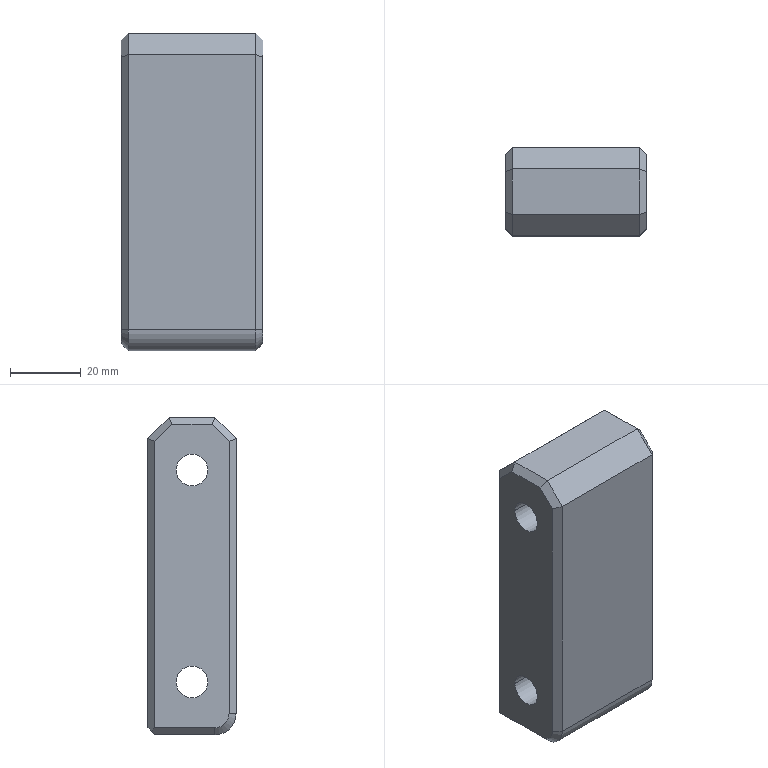Part | Creo | 1 solid | 34 faces | box 40 x 25 x 90 mm | volume 80599 mm3 | plane 23 | cylinder 9 | cone 2 | commonest cylinder face diameters 9 x4 14 x4 12 x1
STEP:
#1=CARTESIAN_POINT('',(294.5,48.167,78.));
#2=VERTEX_POINT('',#1);
#3=CARTESIAN_POINT('',(294.5,52.995,73.172));
#4=VERTEX_POINT('',#3);
#5=CARTESIAN_POINT('',(294.5,48.167,78.));
#6=DIRECTION('',(0.,0.7071,-0.7071));
#7=VECTOR('',#6,6.828);
#8=LINE('',#5,#7);
#9=EDGE_CURVE('',#2,#4,#8,.T.);
#10=ORIENTED_EDGE('',*,*,#9,.F.);
#11=CARTESIAN_POINT('',(294.5,36.824,78.));
#12=VERTEX_POINT('',#11);
#13=CARTESIAN_POINT('',(294.5,48.167,78.));
#14=DIRECTION('',(0.,-1.,0.));
#15=VECTOR('',#14,11.343);
#16=LINE('',#13,#15);
#17=EDGE_CURVE('',#2,#12,#16,.T.);
#18=ORIENTED_EDGE('',*,*,#17,.T.);
#19=CARTESIAN_POINT('',(294.5,31.995,73.172));
#20=VERTEX_POINT('',#19);
#21=CARTESIAN_POINT('',(294.5,31.995,73.172));
#22=DIRECTION('',(0.,0.7071,0.7071));
#23=VECTOR('',#22,6.828);
#24=LINE('',#21,#23);
#25=EDGE_CURVE('',#20,#12,#24,.T.);
#26=ORIENTED_EDGE('',*,*,#25,.F.);
#27=CARTESIAN_POINT('',(294.5,31.995,-4.));
#28=VERTEX_POINT('',#27);
#29=CARTESIAN_POINT('',(294.5,31.995,73.172));
#30=DIRECTION('',(0.,0.,-1.));
#31=VECTOR('',#30,77.172);
#32=LINE('',#29,#31);
#33=EDGE_CURVE('',#20,#28,#32,.T.);
#34=ORIENTED_EDGE('',*,*,#33,.T.);
#35=CARTESIAN_POINT('',(294.5,35.995,-8.));
#36=VERTEX_POINT('',#35);
#37=CARTESIAN_POINT('',(294.5,35.995,-4.));
#38=DIRECTION('',(-1.,0.,0.));
#39=DIRECTION('',(0.,0.,-1.));
#40=AXIS2_PLACEMENT_3D('',#37,#38,#39);
#41=CIRCLE('',#40,4.);
#42=EDGE_CURVE('',#36,#28,#41,.T.);
#43=ORIENTED_EDGE('',*,*,#42,.F.);
#44=CARTESIAN_POINT('',(294.5,52.995,-8.));
#45=VERTEX_POINT('',#44);
#46=CARTESIAN_POINT('',(294.5,35.995,-8.));
#47=DIRECTION('',(0.,1.,0.));
#48=VECTOR('',#47,17.);
#49=LINE('',#46,#48);
#50=EDGE_CURVE('',#36,#45,#49,.T.);
#51=ORIENTED_EDGE('',*,*,#50,.T.);
#52=CARTESIAN_POINT('',(294.5,52.995,-8.));
#53=DIRECTION('',(0.,0.,1.));
#54=VECTOR('',#53,81.172);
#55=LINE('',#52,#54);
#56=EDGE_CURVE('',#45,#4,#55,.T.);
#57=ORIENTED_EDGE('',*,*,#56,.T.);
#58=EDGE_LOOP('',(#10,#18,#26,#34,#43,#51,#57));
#59=FACE_OUTER_BOUND('',#58,.F.);
#60=CARTESIAN_POINT('',(294.5,46.995,65.));
#61=VERTEX_POINT('',#60);
#62=CARTESIAN_POINT('',(294.5,37.995,65.));
#63=VERTEX_POINT('',#62);
#64=CARTESIAN_POINT('',(294.5,42.495,65.));
#65=DIRECTION('',(1.,0.,0.));
#66=DIRECTION('',(0.,1.,0.));
#67=AXIS2_PLACEMENT_3D('',#64,#65,#66);
#68=CIRCLE('',#67,4.5);
#69=EDGE_CURVE('',#61,#63,#68,.T.);
#70=ORIENTED_EDGE('',*,*,#69,.F.);
#71=CARTESIAN_POINT('',(294.5,42.495,65.));
#72=DIRECTION('',(1.,0.,0.));
#73=DIRECTION('',(0.,-1.,0.));
#74=AXIS2_PLACEMENT_3D('',#71,#72,#73);
#75=CIRCLE('',#74,4.5);
#76=EDGE_CURVE('',#63,#61,#75,.T.);
#77=ORIENTED_EDGE('',*,*,#76,.F.);
#78=EDGE_LOOP('',(#70,#77));
#79=FACE_BOUND('',#78,.F.);
#80=CARTESIAN_POINT('',(294.5,46.995,5.));
#81=VERTEX_POINT('',#80);
#82=CARTESIAN_POINT('',(294.5,37.995,5.));
#83=VERTEX_POINT('',#82);
#84=CARTESIAN_POINT('',(294.5,42.495,5.));
#85=DIRECTION('',(1.,0.,0.));
#86=DIRECTION('',(0.,1.,0.));
#87=AXIS2_PLACEMENT_3D('',#84,#85,#86);
#88=CIRCLE('',#87,4.5);
#89=EDGE_CURVE('',#81,#83,#88,.T.);
#90=ORIENTED_EDGE('',*,*,#89,.F.);
#91=CARTESIAN_POINT('',(294.5,42.495,5.));
#92=DIRECTION('',(1.,0.,0.));
#93=DIRECTION('',(0.,-1.,0.));
#94=AXIS2_PLACEMENT_3D('',#91,#92,#93);
#95=CIRCLE('',#94,4.5);
#96=EDGE_CURVE('',#83,#81,#95,.T.);
#97=ORIENTED_EDGE('',*,*,#96,.F.);
#98=EDGE_LOOP('',(#90,#97));
#99=FACE_BOUND('',#98,.F.);
#100=CARTESIAN_POINT('',(294.5,42.745,-10.));
#101=DIRECTION('',(-1.,0.,0.));
#102=DIRECTION('',(0.,0.,-1.));
#103=AXIS2_PLACEMENT_3D('',#100,#101,#102);
#104=PLANE('',#103);
#105=ADVANCED_FACE('',(#59,#79,#99),#104,.T.);
#106=ORIENTED_EDGE('',*,*,#69,.T.);
#107=CARTESIAN_POINT('',(325.5,37.995,65.));
#108=VERTEX_POINT('',#107);
#109=CARTESIAN_POINT('',(294.5,37.995,65.));
#110=DIRECTION('',(1.,0.,0.));
#111=VECTOR('',#110,31.);
#112=LINE('',#109,#111);
#113=EDGE_CURVE('',#63,#108,#112,.T.);
#114=ORIENTED_EDGE('',*,*,#113,.T.);
#115=CARTESIAN_POINT('',(325.5,46.995,65.));
#116=VERTEX_POINT('',#115);
#117=CARTESIAN_POINT('',(325.5,42.495,65.));
#118=DIRECTION('',(-1.,0.,0.));
#119=DIRECTION('',(0.,-1.,0.));
#120=AXIS2_PLACEMENT_3D('',#117,#118,#119);
#121=CIRCLE('',#120,4.5);
#122=EDGE_CURVE('',#108,#116,#121,.T.);
#123=ORIENTED_EDGE('',*,*,#122,.T.);
#124=CARTESIAN_POINT('',(294.5,46.995,65.));
#125=DIRECTION('',(1.,0.,0.));
#126=VECTOR('',#125,31.);
#127=LINE('',#124,#126);
#128=EDGE_CURVE('',#61,#116,#127,.T.);
#129=ORIENTED_EDGE('',*,*,#128,.F.);
#130=EDGE_LOOP('',(#106,#114,#123,#129));
#131=FACE_OUTER_BOUND('',#130,.F.);
#132=CARTESIAN_POINT('',(334.5,42.495,65.));
#133=DIRECTION('',(1.,0.,0.));
#134=DIRECTION('',(0.,1.,0.));
#135=AXIS2_PLACEMENT_3D('',#132,#133,#134);
#136=CYLINDRICAL_SURFACE('',#135,4.5);
#137=ADVANCED_FACE('',(#131),#136,.F.);
#138=ORIENTED_EDGE('',*,*,#76,.T.);
#139=ORIENTED_EDGE('',*,*,#128,.T.);
#140=CARTESIAN_POINT('',(325.5,42.495,65.));
#141=DIRECTION('',(-1.,0.,0.));
#142=DIRECTION('',(0.,1.,0.));
#143=AXIS2_PLACEMENT_3D('',#140,#141,#142);
#144=CIRCLE('',#143,4.5);
#145=EDGE_CURVE('',#116,#108,#144,.T.);
#146=ORIENTED_EDGE('',*,*,#145,.T.);
#147=ORIENTED_EDGE('',*,*,#113,.F.);
#148=EDGE_LOOP('',(#138,#139,#146,#147));
#149=FACE_OUTER_BOUND('',#148,.F.);
#150=CARTESIAN_POINT('',(334.5,42.495,65.));
#151=DIRECTION('',(1.,0.,0.));
#152=DIRECTION('',(0.,1.,0.));
#153=AXIS2_PLACEMENT_3D('',#150,#151,#152);
#154=CYLINDRICAL_SURFACE('',#153,4.5);
#155=ADVANCED_FACE('',(#149),#154,.F.);
#156=CARTESIAN_POINT('',(325.5,49.495,65.));
#157=VERTEX_POINT('',#156);
#158=CARTESIAN_POINT('',(325.5,35.495,65.));
#159=VERTEX_POINT('',#158);
#160=CARTESIAN_POINT('',(325.5,42.495,65.));
#161=DIRECTION('',(1.,0.,0.));
#162=DIRECTION('',(0.,1.,0.));
#163=AXIS2_PLACEMENT_3D('',#160,#161,#162);
#164=CIRCLE('',#163,7.);
#165=EDGE_CURVE('',#157,#159,#164,.T.);
#166=ORIENTED_EDGE('',*,*,#165,.F.);
#167=CARTESIAN_POINT('',(325.5,42.495,65.));
#168=DIRECTION('',(1.,0.,0.));
#169=DIRECTION('',(0.,-1.,0.));
#170=AXIS2_PLACEMENT_3D('',#167,#168,#169);
#171=CIRCLE('',#170,7.);
#172=EDGE_CURVE('',#159,#157,#171,.T.);
#173=ORIENTED_EDGE('',*,*,#172,.F.);
#174=EDGE_LOOP('',(#166,#173));
#175=FACE_OUTER_BOUND('',#174,.F.);
#176=ORIENTED_EDGE('',*,*,#145,.F.);
#177=ORIENTED_EDGE('',*,*,#122,.F.);
#178=EDGE_LOOP('',(#176,#177));
#179=FACE_BOUND('',#178,.F.);
#180=CARTESIAN_POINT('',(325.5,42.495,65.));
#181=DIRECTION('',(-1.,0.,0.));
#182=DIRECTION('',(0.,0.,1.));
#183=AXIS2_PLACEMENT_3D('',#180,#181,#182);
#184=PLANE('',#183);
#185=ADVANCED_FACE('',(#175,#179),#184,.F.);
#186=ORIENTED_EDGE('',*,*,#165,.T.);
#187=CARTESIAN_POINT('',(334.5,35.495,65.));
#188=VERTEX_POINT('',#187);
#189=CARTESIAN_POINT('',(334.5,35.495,65.));
#190=DIRECTION('',(-1.,0.,0.));
#191=VECTOR('',#190,9.);
#192=LINE('',#189,#191);
#193=EDGE_CURVE('',#188,#159,#192,.T.);
#194=ORIENTED_EDGE('',*,*,#193,.F.);
#195=CARTESIAN_POINT('',(334.5,49.495,65.));
#196=VERTEX_POINT('',#195);
#197=CARTESIAN_POINT('',(334.5,42.495,65.));
#198=DIRECTION('',(-1.,0.,0.));
#199=DIRECTION('',(0.,-1.,0.));
#200=AXIS2_PLACEMENT_3D('',#197,#198,#199);
#201=CIRCLE('',#200,7.);
#202=EDGE_CURVE('',#188,#196,#201,.T.);
#203=ORIENTED_EDGE('',*,*,#202,.T.);
#204=CARTESIAN_POINT('',(334.5,49.495,65.));
#205=DIRECTION('',(-1.,0.,0.));
#206=VECTOR('',#205,9.);
#207=LINE('',#204,#206);
#208=EDGE_CURVE('',#196,#157,#207,.T.);
#209=ORIENTED_EDGE('',*,*,#208,.T.);
#210=EDGE_LOOP('',(#186,#194,#203,#209));
#211=FACE_OUTER_BOUND('',#210,.F.);
#212=CARTESIAN_POINT('',(334.5,42.495,65.));
#213=DIRECTION('',(-1.,0.,0.));
#214=DIRECTION('',(0.,1.,0.));
#215=AXIS2_PLACEMENT_3D('',#212,#213,#214);
#216=CYLINDRICAL_SURFACE('',#215,7.);
#217=ADVANCED_FACE('',(#211),#216,.F.);
#218=ORIENTED_EDGE('',*,*,#172,.T.);
#219=ORIENTED_EDGE('',*,*,#208,.F.);
#220=CARTESIAN_POINT('',(334.5,42.495,65.));
#221=DIRECTION('',(-1.,0.,0.));
#222=DIRECTION('',(0.,1.,0.));
#223=AXIS2_PLACEMENT_3D('',#220,#221,#222);
#224=CIRCLE('',#223,7.);
#225=EDGE_CURVE('',#196,#188,#224,.T.);
#226=ORIENTED_EDGE('',*,*,#225,.T.);
#227=ORIENTED_EDGE('',*,*,#193,.T.);
#228=EDGE_LOOP('',(#218,#219,#226,#227));
#229=FACE_OUTER_BOUND('',#228,.F.);
#230=CARTESIAN_POINT('',(334.5,42.495,65.));
#231=DIRECTION('',(-1.,0.,0.));
#232=DIRECTION('',(0.,1.,0.));
#233=AXIS2_PLACEMENT_3D('',#230,#231,#232);
#234=CYLINDRICAL_SURFACE('',#233,7.);
#235=ADVANCED_FACE('',(#229),#234,.F.);
#236=CARTESIAN_POINT('',(334.5,52.995,73.172));
#237=VERTEX_POINT('',#236);
#238=CARTESIAN_POINT('',(334.5,48.167,78.));
#239=VERTEX_POINT('',#238);
#240=CARTESIAN_POINT('',(334.5,52.995,73.172));
#241=DIRECTION('',(0.,-0.7071,0.7071));
#242=VECTOR('',#241,6.828);
#243=LINE('',#240,#242);
#244=EDGE_CURVE('',#237,#239,#243,.T.);
#245=ORIENTED_EDGE('',*,*,#244,.F.);
#246=CARTESIAN_POINT('',(334.5,52.995,-8.));
#247=VERTEX_POINT('',#246);
#248=CARTESIAN_POINT('',(334.5,52.995,73.172));
#249=DIRECTION('',(0.,0.,-1.));
#250=VECTOR('',#249,81.172);
#251=LINE('',#248,#250);
#252=EDGE_CURVE('',#237,#247,#251,.T.);
#253=ORIENTED_EDGE('',*,*,#252,.T.);
#254=CARTESIAN_POINT('',(334.5,35.995,-8.));
#255=VERTEX_POINT('',#254);
#256=CARTESIAN_POINT('',(334.5,52.995,-8.));
#257=DIRECTION('',(0.,-1.,0.));
#258=VECTOR('',#257,17.);
#259=LINE('',#256,#258);
#260=EDGE_CURVE('',#247,#255,#259,.T.);
#261=ORIENTED_EDGE('',*,*,#260,.T.);
#262=CARTESIAN_POINT('',(334.5,31.995,-4.));
#263=VERTEX_POINT('',#262);
#264=CARTESIAN_POINT('',(334.5,35.995,-4.));
#265=DIRECTION('',(1.,0.,0.));
#266=DIRECTION('',(0.,-1.,0.));
#267=AXIS2_PLACEMENT_3D('',#264,#265,#266);
#268=CIRCLE('',#267,4.);
#269=EDGE_CURVE('',#263,#255,#268,.T.);
#270=ORIENTED_EDGE('',*,*,#269,.F.);
#271=CARTESIAN_POINT('',(334.5,31.995,73.172));
#272=VERTEX_POINT('',#271);
#273=CARTESIAN_POINT('',(334.5,31.995,-4.));
#274=DIRECTION('',(0.,0.,1.));
#275=VECTOR('',#274,77.172);
#276=LINE('',#273,#275);
#277=EDGE_CURVE('',#263,#272,#276,.T.);
#278=ORIENTED_EDGE('',*,*,#277,.T.);
#279=CARTESIAN_POINT('',(334.5,36.824,78.));
#280=VERTEX_POINT('',#279);
#281=CARTESIAN_POINT('',(334.5,36.824,78.));
#282=DIRECTION('',(0.,-0.7071,-0.7071));
#283=VECTOR('',#282,6.828);
#284=LINE('',#281,#283);
#285=EDGE_CURVE('',#280,#272,#284,.T.);
#286=ORIENTED_EDGE('',*,*,#285,.F.);
#287=CARTESIAN_POINT('',(334.5,36.824,78.));
#288=DIRECTION('',(0.,1.,0.));
#289=VECTOR('',#288,11.343);
#290=LINE('',#287,#289);
#291=EDGE_CURVE('',#280,#239,#290,.T.);
#292=ORIENTED_EDGE('',*,*,#291,.T.);
#293=EDGE_LOOP('',(#245,#253,#261,#270,#278,#286,#292));
#294=FACE_OUTER_BOUND('',#293,.F.);
#295=ORIENTED_EDGE('',*,*,#225,.F.);
#296=ORIENTED_EDGE('',*,*,#202,.F.);
#297=EDGE_LOOP('',(#295,#296));
#298=FACE_BOUND('',#297,.F.);
#299=CARTESIAN_POINT('',(334.5,49.495,5.));
#300=VERTEX_POINT('',#299);
#301=CARTESIAN_POINT('',(334.5,35.495,5.));
#302=VERTEX_POINT('',#301);
#303=CARTESIAN_POINT('',(334.5,42.495,5.));
#304=DIRECTION('',(-1.,0.,0.));
#305=DIRECTION('',(0.,1.,0.));
#306=AXIS2_PLACEMENT_3D('',#303,#304,#305);
#307=CIRCLE('',#306,7.);
#308=EDGE_CURVE('',#300,#302,#307,.T.);
#309=ORIENTED_EDGE('',*,*,#308,.F.);
#310=CARTESIAN_POINT('',(334.5,42.495,5.));
#311=DIRECTION('',(-1.,0.,0.));
#312=DIRECTION('',(0.,-1.,0.));
#313=AXIS2_PLACEMENT_3D('',#310,#311,#312);
#314=CIRCLE('',#313,7.);
#315=EDGE_CURVE('',#302,#300,#314,.T.);
#316=ORIENTED_EDGE('',*,*,#315,.F.);
#317=EDGE_LOOP('',(#309,#316));
#318=FACE_BOUND('',#317,.F.);
#319=CARTESIAN_POINT('',(334.5,42.745,-10.));
#320=DIRECTION('',(1.,0.,0.));
#321=DIRECTION('',(0.,0.,1.));
#322=AXIS2_PLACEMENT_3D('',#319,#320,#321);
#323=PLANE('',#322);
#324=ADVANCED_FACE('',(#294,#298,#318),#323,.T.);
#325=CARTESIAN_POINT('',(332.5,54.995,74.));
#326=VERTEX_POINT('',#325);
#327=CARTESIAN_POINT('',(332.5,54.995,74.));
#328=DIRECTION('',(0.6786,-0.6786,-0.2811));
#329=VECTOR('',#328,2.947);
#330=LINE('',#327,#329);
#331=EDGE_CURVE('',#326,#237,#330,.T.);
#332=ORIENTED_EDGE('',*,*,#331,.T.);
#333=ORIENTED_EDGE('',*,*,#244,.T.);
#334=CARTESIAN_POINT('',(332.5,48.995,80.));
#335=VERTEX_POINT('',#334);
#336=CARTESIAN_POINT('',(334.5,48.167,78.));
#337=DIRECTION('',(-0.6786,0.2811,0.6786));
#338=VECTOR('',#337,2.947);
#339=LINE('',#336,#338);
#340=EDGE_CURVE('',#239,#335,#339,.T.);
#341=ORIENTED_EDGE('',*,*,#340,.T.);
#342=CARTESIAN_POINT('',(332.5,54.995,74.));
#343=DIRECTION('',(0.,-0.7071,0.7071));
#344=VECTOR('',#343,8.485);
#345=LINE('',#342,#344);
#346=EDGE_CURVE('',#326,#335,#345,.T.);
#347=ORIENTED_EDGE('',*,*,#346,.F.);
#348=EDGE_LOOP('',(#332,#333,#341,#347));
#349=FACE_OUTER_BOUND('',#348,.F.);
#350=CARTESIAN_POINT('',(334.5,89.456,36.711));
#351=DIRECTION('',(0.7071,0.5,0.5));
#352=DIRECTION('',(0.,0.7071,-0.7071));
#353=AXIS2_PLACEMENT_3D('',#350,#351,#352);
#354=PLANE('',#353);
#355=ADVANCED_FACE('',(#349),#354,.T.);
#356=CARTESIAN_POINT('',(333.5,53.995,-9.));
#357=VERTEX_POINT('',#356);
#358=CARTESIAN_POINT('',(333.5,53.995,-9.));
#359=DIRECTION('',(0.5774,-0.5774,0.5774));
#360=VECTOR('',#359,1.732);
#361=LINE('',#358,#360);
#362=EDGE_CURVE('',#357,#247,#361,.T.);
#363=ORIENTED_EDGE('',*,*,#362,.T.);
#364=ORIENTED_EDGE('',*,*,#252,.F.);
#365=ORIENTED_EDGE('',*,*,#331,.F.);
#366=CARTESIAN_POINT('',(332.5,54.995,-8.));
#367=VERTEX_POINT('',#366);
#368=CARTESIAN_POINT('',(332.5,54.995,-8.));
#369=DIRECTION('',(0.,0.,1.));
#370=VECTOR('',#369,82.);
#371=LINE('',#368,#370);
#372=EDGE_CURVE('',#367,#326,#371,.T.);
#373=ORIENTED_EDGE('',*,*,#372,.F.);
#374=CARTESIAN_POINT('',(332.5,54.995,-8.));
#375=DIRECTION('',(0.5774,-0.5774,-0.5774));
#376=VECTOR('',#375,1.732);
#377=LINE('',#374,#376);
#378=EDGE_CURVE('',#367,#357,#377,.T.);
#379=ORIENTED_EDGE('',*,*,#378,.T.);
#380=EDGE_LOOP('',(#363,#364,#365,#373,#379));
#381=FACE_OUTER_BOUND('',#380,.F.);
#382=CARTESIAN_POINT('',(332.5,54.995,35.));
#383=DIRECTION('',(0.7071,0.7071,0.));
#384=DIRECTION('',(0.,0.,1.));
#385=AXIS2_PLACEMENT_3D('',#382,#383,#384);
#386=PLANE('',#385);
#387=ADVANCED_FACE('',(#381),#386,.T.);
#388=CARTESIAN_POINT('',(332.5,35.995,-10.));
#389=VERTEX_POINT('',#388);
#390=CARTESIAN_POINT('',(332.5,52.995,-10.));
#391=VERTEX_POINT('',#390);
#392=CARTESIAN_POINT('',(332.5,35.995,-10.));
#393=DIRECTION('',(0.,1.,0.));
#394=VECTOR('',#393,17.);
#395=LINE('',#392,#394);
#396=EDGE_CURVE('',#389,#391,#395,.T.);
#397=ORIENTED_EDGE('',*,*,#396,.F.);
#398=CARTESIAN_POINT('',(332.5,35.995,-10.));
#399=DIRECTION('',(0.7071,0.,0.7071));
#400=VECTOR('',#399,2.828);
#401=LINE('',#398,#400);
#402=EDGE_CURVE('',#389,#255,#401,.T.);
#403=ORIENTED_EDGE('',*,*,#402,.T.);
#404=ORIENTED_EDGE('',*,*,#260,.F.);
#405=ORIENTED_EDGE('',*,*,#362,.F.);
#406=CARTESIAN_POINT('',(333.5,53.995,-9.));
#407=DIRECTION('',(-0.5774,-0.5774,-0.5774));
#408=VECTOR('',#407,1.732);
#409=LINE('',#406,#408);
#410=EDGE_CURVE('',#357,#391,#409,.T.);
#411=ORIENTED_EDGE('',*,*,#410,.T.);
#412=EDGE_LOOP('',(#397,#403,#404,#405,#411));
#413=FACE_OUTER_BOUND('',#412,.F.);
#414=CARTESIAN_POINT('',(332.5,42.745,-10.));
#415=DIRECTION('',(-0.7071,0.,0.7071));
#416=DIRECTION('',(0.,-1.,0.));
#417=AXIS2_PLACEMENT_3D('',#414,#415,#416);
#418=PLANE('',#417);
#419=ADVANCED_FACE('',(#413),#418,.F.);
#420=CARTESIAN_POINT('',(296.5,52.995,-10.));
#421=VERTEX_POINT('',#420);
#422=CARTESIAN_POINT('',(296.5,35.995,-10.));
#423=VERTEX_POINT('',#422);
#424=CARTESIAN_POINT('',(296.5,52.995,-10.));
#425=DIRECTION('',(0.,-1.,0.));
#426=VECTOR('',#425,17.);
#427=LINE('',#424,#426);
#428=EDGE_CURVE('',#421,#423,#427,.T.);
#429=ORIENTED_EDGE('',*,*,#428,.T.);
#430=CARTESIAN_POINT('',(296.5,35.995,-10.));
#431=DIRECTION('',(1.,0.,0.));
#432=VECTOR('',#431,36.);
#433=LINE('',#430,#432);
#434=EDGE_CURVE('',#423,#389,#433,.T.);
#435=ORIENTED_EDGE('',*,*,#434,.T.);
#436=ORIENTED_EDGE('',*,*,#396,.T.);
#437=CARTESIAN_POINT('',(332.5,52.995,-10.));
#438=DIRECTION('',(-1.,0.,0.));
#439=VECTOR('',#438,36.);
#440=LINE('',#437,#439);
#441=EDGE_CURVE('',#391,#421,#440,.T.);
#442=ORIENTED_EDGE('',*,*,#441,.T.);
#443=EDGE_LOOP('',(#429,#435,#436,#442));
#444=FACE_OUTER_BOUND('',#443,.F.);
#445=CARTESIAN_POINT('',(318.5,42.745,-10.));
#446=DIRECTION('',(0.,0.,-1.));
#447=DIRECTION('',(1.,0.,0.));
#448=AXIS2_PLACEMENT_3D('',#445,#446,#447);
#449=PLANE('',#448);
#450=ADVANCED_FACE('',(#444),#449,.T.);
#451=CARTESIAN_POINT('',(295.5,53.995,-9.));
#452=VERTEX_POINT('',#451);
#453=CARTESIAN_POINT('',(294.5,52.995,-8.));
#454=DIRECTION('',(0.5774,0.5774,-0.5774));
#455=VECTOR('',#454,1.732);
#456=LINE('',#453,#455);
#457=EDGE_CURVE('',#45,#452,#456,.T.);
#458=ORIENTED_EDGE('',*,*,#457,.F.);
#459=ORIENTED_EDGE('',*,*,#50,.F.);
#460=CARTESIAN_POINT('',(294.5,35.995,-8.));
#461=DIRECTION('',(0.7071,0.,-0.7071));
#462=VECTOR('',#461,2.828);
#463=LINE('',#460,#462);
#464=EDGE_CURVE('',#36,#423,#463,.T.);
#465=ORIENTED_EDGE('',*,*,#464,.T.);
#466=ORIENTED_EDGE('',*,*,#428,.F.);
#467=CARTESIAN_POINT('',(296.5,52.995,-10.));
#468=DIRECTION('',(-0.5774,0.5774,0.5774));
#469=VECTOR('',#468,1.732);
#470=LINE('',#467,#469);
#471=EDGE_CURVE('',#421,#452,#470,.T.);
#472=ORIENTED_EDGE('',*,*,#471,.T.);
#473=EDGE_LOOP('',(#458,#459,#465,#466,#472));
#474=FACE_OUTER_BOUND('',#473,.F.);
#475=CARTESIAN_POINT('',(296.5,42.745,-10.));
#476=DIRECTION('',(0.7071,0.,0.7071));
#477=DIRECTION('',(0.,1.,0.));
#478=AXIS2_PLACEMENT_3D('',#475,#476,#477);
#479=PLANE('',#478);
#480=ADVANCED_FACE('',(#474),#479,.F.);
#481=CARTESIAN_POINT('',(296.5,54.995,74.));
#482=VERTEX_POINT('',#481);
#483=CARTESIAN_POINT('',(296.5,54.995,-8.));
#484=VERTEX_POINT('',#483);
#485=CARTESIAN_POINT('',(296.5,54.995,74.));
#486=DIRECTION('',(0.,0.,-1.));
#487=VECTOR('',#486,82.);
#488=LINE('',#485,#487);
#489=EDGE_CURVE('',#482,#484,#488,.T.);
#490=ORIENTED_EDGE('',*,*,#489,.F.);
#491=CARTESIAN_POINT('',(296.5,54.995,74.));
#492=DIRECTION('',(-0.6786,-0.6786,-0.2811));
#493=VECTOR('',#492,2.947);
#494=LINE('',#491,#493);
#495=EDGE_CURVE('',#482,#4,#494,.T.);
#496=ORIENTED_EDGE('',*,*,#495,.T.);
#497=ORIENTED_EDGE('',*,*,#56,.F.);
#498=ORIENTED_EDGE('',*,*,#457,.T.);
#499=CARTESIAN_POINT('',(295.5,53.995,-9.));
#500=DIRECTION('',(0.5774,0.5774,0.5774));
#501=VECTOR('',#500,1.732);
#502=LINE('',#499,#501);
#503=EDGE_CURVE('',#452,#484,#502,.T.);
#504=ORIENTED_EDGE('',*,*,#503,.T.);
#505=EDGE_LOOP('',(#490,#496,#497,#498,#504));
#506=FACE_OUTER_BOUND('',#505,.F.);
#507=CARTESIAN_POINT('',(294.5,52.995,-10.));
#508=DIRECTION('',(-0.7071,0.7071,0.));
#509=DIRECTION('',(0.,0.,1.));
#510=AXIS2_PLACEMENT_3D('',#507,#508,#509);
#511=PLANE('',#510);
#512=ADVANCED_FACE('',(#506),#511,.T.);
#513=ORIENTED_EDGE('',*,*,#372,.T.);
#514=CARTESIAN_POINT('',(332.5,54.995,74.));
#515=DIRECTION('',(-1.,0.,0.));
#516=VECTOR('',#515,36.);
#517=LINE('',#514,#516);
#518=EDGE_CURVE('',#326,#482,#517,.T.);
#519=ORIENTED_EDGE('',*,*,#518,.T.);
#520=ORIENTED_EDGE('',*,*,#489,.T.);
#521=CARTESIAN_POINT('',(296.5,54.995,-8.));
#522=DIRECTION('',(1.,0.,0.));
#523=VECTOR('',#522,36.);
#524=LINE('',#521,#523);
#525=EDGE_CURVE('',#484,#367,#524,.T.);
#526=ORIENTED_EDGE('',*,*,#525,.T.);
#527=EDGE_LOOP('',(#513,#519,#520,#526));
#528=FACE_OUTER_BOUND('',#527,.F.);
#529=CARTESIAN_POINT('',(318.5,54.995,35.));
#530=DIRECTION('',(0.,-1.,0.));
#531=DIRECTION('',(0.,0.,-1.));
#532=AXIS2_PLACEMENT_3D('',#529,#530,#531);
#533=PLANE('',#532);
#534=ADVANCED_FACE('',(#528),#533,.F.);
#535=CARTESIAN_POINT('',(296.5,48.995,80.));
#536=VERTEX_POINT('',#535);
#537=CARTESIAN_POINT('',(296.5,48.995,80.));
#538=DIRECTION('',(1.,0.,0.));
#539=VECTOR('',#538,36.);
#540=LINE('',#537,#539);
#541=EDGE_CURVE('',#536,#335,#540,.T.);
#542=ORIENTED_EDGE('',*,*,#541,.F.);
#543=CARTESIAN_POINT('',(296.5,48.995,80.));
#544=DIRECTION('',(0.,0.7071,-0.7071));
#545=VECTOR('',#544,8.485);
#546=LINE('',#543,#545);
#547=EDGE_CURVE('',#536,#482,#546,.T.);
#548=ORIENTED_EDGE('',*,*,#547,.T.);
#549=ORIENTED_EDGE('',*,*,#518,.F.);
#550=ORIENTED_EDGE('',*,*,#346,.T.);
#551=EDGE_LOOP('',(#542,#548,#549,#550));
#552=FACE_OUTER_BOUND('',#551,.F.);
#553=CARTESIAN_POINT('',(318.5,54.995,74.));
#554=DIRECTION('',(0.,-0.7071,-0.7071));
#555=DIRECTION('',(1.,0.,0.));
#556=AXIS2_PLACEMENT_3D('',#553,#554,#555);
#557=PLANE('',#556);
#558=ADVANCED_FACE('',(#552),#557,.F.);
#559=CARTESIAN_POINT('',(332.5,35.995,80.));
#560=VERTEX_POINT('',#559);
#561=CARTESIAN_POINT('',(296.5,35.995,80.));
#562=VERTEX_POINT('',#561);
#563=CARTESIAN_POINT('',(332.5,35.995,80.));
#564=DIRECTION('',(-1.,0.,0.));
#565=VECTOR('',#564,36.);
#566=LINE('',#563,#565);
#567=EDGE_CURVE('',#560,#562,#566,.T.);
#568=ORIENTED_EDGE('',*,*,#567,.T.);
#569=CARTESIAN_POINT('',(296.5,35.995,80.));
#570=DIRECTION('',(0.,1.,0.));
#571=VECTOR('',#570,13.);
#572=LINE('',#569,#571);
#573=EDGE_CURVE('',#562,#536,#572,.T.);
#574=ORIENTED_EDGE('',*,*,#573,.T.);
#575=ORIENTED_EDGE('',*,*,#541,.T.);
#576=CARTESIAN_POINT('',(332.5,48.995,80.));
#577=DIRECTION('',(0.,-1.,0.));
#578=VECTOR('',#577,13.);
#579=LINE('',#576,#578);
#580=EDGE_CURVE('',#335,#560,#579,.T.);
#581=ORIENTED_EDGE('',*,*,#580,.T.);
#582=EDGE_LOOP('',(#568,#574,#575,#581));
#583=FACE_OUTER_BOUND('',#582,.F.);
#584=CARTESIAN_POINT('',(318.5,42.745,80.));
#585=DIRECTION('',(0.,0.,-1.));
#586=DIRECTION('',(1.,0.,0.));
#587=AXIS2_PLACEMENT_3D('',#584,#585,#586);
#588=PLANE('',#587);
#589=ADVANCED_FACE('',(#583),#588,.F.);
#590=CARTESIAN_POINT('',(296.5,29.995,74.));
#591=VERTEX_POINT('',#590);
#592=CARTESIAN_POINT('',(332.5,29.995,74.));
#593=VERTEX_POINT('',#592);
#594=CARTESIAN_POINT('',(296.5,29.995,74.));
#595=DIRECTION('',(1.,0.,0.));
#596=VECTOR('',#595,36.);
#597=LINE('',#594,#596);
#598=EDGE_CURVE('',#591,#593,#597,.T.);
#599=ORIENTED_EDGE('',*,*,#598,.F.);
#600=CARTESIAN_POINT('',(296.5,29.995,74.));
#601=DIRECTION('',(0.,0.7071,0.7071));
#602=VECTOR('',#601,8.485);
#603=LINE('',#600,#602);
#604=EDGE_CURVE('',#591,#562,#603,.T.);
#605=ORIENTED_EDGE('',*,*,#604,.T.);
#606=ORIENTED_EDGE('',*,*,#567,.F.);
#607=CARTESIAN_POINT('',(332.5,35.995,80.));
#608=DIRECTION('',(0.,-0.7071,-0.7071));
#609=VECTOR('',#608,8.485);
#610=LINE('',#607,#609);
#611=EDGE_CURVE('',#560,#593,#610,.T.);
#612=ORIENTED_EDGE('',*,*,#611,.T.);
#613=EDGE_LOOP('',(#599,#605,#606,#612));
#614=FACE_OUTER_BOUND('',#613,.F.);
#615=CARTESIAN_POINT('',(318.5,35.995,80.));
#616=DIRECTION('',(0.,-0.7071,0.7071));
#617=DIRECTION('',(-1.,0.,0.));
#618=AXIS2_PLACEMENT_3D('',#615,#616,#617);
#619=PLANE('',#618);
#620=ADVANCED_FACE('',(#614),#619,.T.);
#621=CARTESIAN_POINT('',(332.5,29.995,-4.));
#622=VERTEX_POINT('',#621);
#623=CARTESIAN_POINT('',(296.5,29.995,-4.));
#624=VERTEX_POINT('',#623);
#625=CARTESIAN_POINT('',(332.5,29.995,-4.));
#626=DIRECTION('',(-1.,0.,0.));
#627=VECTOR('',#626,36.);
#628=LINE('',#625,#627);
#629=EDGE_CURVE('',#622,#624,#628,.T.);
#630=ORIENTED_EDGE('',*,*,#629,.T.);
#631=CARTESIAN_POINT('',(296.5,29.995,-4.));
#632=DIRECTION('',(0.,0.,1.));
#633=VECTOR('',#632,78.);
#634=LINE('',#631,#633);
#635=EDGE_CURVE('',#624,#591,#634,.T.);
#636=ORIENTED_EDGE('',*,*,#635,.T.);
#637=ORIENTED_EDGE('',*,*,#598,.T.);
#638=CARTESIAN_POINT('',(332.5,29.995,74.));
#639=DIRECTION('',(0.,0.,-1.));
#640=VECTOR('',#639,78.);
#641=LINE('',#638,#640);
#642=EDGE_CURVE('',#593,#622,#641,.T.);
#643=ORIENTED_EDGE('',*,*,#642,.T.);
#644=EDGE_LOOP('',(#630,#636,#637,#643));
#645=FACE_OUTER_BOUND('',#644,.F.);
#646=CARTESIAN_POINT('',(318.5,29.995,-10.));
#647=DIRECTION('',(0.,-1.,0.));
#648=DIRECTION('',(0.,0.,-1.));
#649=AXIS2_PLACEMENT_3D('',#646,#647,#648);
#650=PLANE('',#649);
#651=ADVANCED_FACE('',(#645),#650,.T.);
#652=ORIENTED_EDGE('',*,*,#434,.F.);
#653=CARTESIAN_POINT('',(296.5,35.995,-4.));
#654=DIRECTION('',(-1.,0.,0.));
#655=DIRECTION('',(0.,0.,-1.));
#656=AXIS2_PLACEMENT_3D('',#653,#654,#655);
#657=CIRCLE('',#656,6.);
#658=EDGE_CURVE('',#423,#624,#657,.T.);
#659=ORIENTED_EDGE('',*,*,#658,.T.);
#660=ORIENTED_EDGE('',*,*,#629,.F.);
#661=CARTESIAN_POINT('',(332.5,35.995,-4.));
#662=DIRECTION('',(1.,0.,0.));
#663=DIRECTION('',(0.,-1.,0.));
#664=AXIS2_PLACEMENT_3D('',#661,#662,#663);
#665=CIRCLE('',#664,6.);
#666=EDGE_CURVE('',#622,#389,#665,.T.);
#667=ORIENTED_EDGE('',*,*,#666,.T.);
#668=EDGE_LOOP('',(#652,#659,#660,#667));
#669=FACE_OUTER_BOUND('',#668,.F.);
#670=CARTESIAN_POINT('',(318.5,35.995,-4.));
#671=DIRECTION('',(-1.,0.,0.));
#672=DIRECTION('',(0.,0.,1.));
#673=AXIS2_PLACEMENT_3D('',#670,#671,#672);
#674=CYLINDRICAL_SURFACE('',#673,6.);
#675=ADVANCED_FACE('',(#669),#674,.T.);
#676=CARTESIAN_POINT('',(296.5,29.995,-4.));
#677=DIRECTION('',(-0.7071,0.7071,0.));
#678=VECTOR('',#677,2.828);
#679=LINE('',#676,#678);
#680=EDGE_CURVE('',#624,#28,#679,.T.);
#681=ORIENTED_EDGE('',*,*,#680,.F.);
#682=ORIENTED_EDGE('',*,*,#658,.F.);
#683=ORIENTED_EDGE('',*,*,#464,.F.);
#684=ORIENTED_EDGE('',*,*,#42,.T.);
#685=EDGE_LOOP('',(#681,#682,#683,#684));
#686=FACE_OUTER_BOUND('',#685,.F.);
#687=CARTESIAN_POINT('',(295.5,35.995,-4.));
#688=DIRECTION('',(1.,0.,0.));
#689=DIRECTION('',(0.,0.,-1.));
#690=AXIS2_PLACEMENT_3D('',#687,#688,#689);
#691=CONICAL_SURFACE('',#690,5.,45.);
#692=ADVANCED_FACE('',(#686),#691,.T.);
#693=CARTESIAN_POINT('',(294.5,31.995,73.172));
#694=DIRECTION('',(0.6786,-0.6786,0.2811));
#695=VECTOR('',#694,2.947);
#696=LINE('',#693,#695);
#697=EDGE_CURVE('',#20,#591,#696,.T.);
#698=ORIENTED_EDGE('',*,*,#697,.T.);
#699=ORIENTED_EDGE('',*,*,#635,.F.);
#700=ORIENTED_EDGE('',*,*,#680,.T.);
#701=ORIENTED_EDGE('',*,*,#33,.F.);
#702=EDGE_LOOP('',(#698,#699,#700,#701));
#703=FACE_OUTER_BOUND('',#702,.F.);
#704=CARTESIAN_POINT('',(296.5,29.995,-10.));
#705=DIRECTION('',(0.7071,0.7071,0.));
#706=DIRECTION('',(0.,0.,-1.));
#707=AXIS2_PLACEMENT_3D('',#704,#705,#706);
#708=PLANE('',#707);
#709=ADVANCED_FACE('',(#703),#708,.F.);
#710=CARTESIAN_POINT('',(296.5,35.995,80.));
#711=DIRECTION('',(-0.6786,0.2811,-0.6786));
#712=VECTOR('',#711,2.947);
#713=LINE('',#710,#712);
#714=EDGE_CURVE('',#562,#12,#713,.T.);
#715=ORIENTED_EDGE('',*,*,#714,.F.);
#716=ORIENTED_EDGE('',*,*,#604,.F.);
#717=ORIENTED_EDGE('',*,*,#697,.F.);
#718=ORIENTED_EDGE('',*,*,#25,.T.);
#719=EDGE_LOOP('',(#715,#716,#717,#718));
#720=FACE_OUTER_BOUND('',#719,.F.);
#721=CARTESIAN_POINT('',(294.5,-4.215,36.961));
#722=DIRECTION('',(0.7071,0.5,-0.5));
#723=DIRECTION('',(0.,0.7071,0.7071));
#724=AXIS2_PLACEMENT_3D('',#721,#722,#723);
#725=PLANE('',#724);
#726=ADVANCED_FACE('',(#720),#725,.F.);
#727=ORIENTED_EDGE('',*,*,#714,.T.);
#728=ORIENTED_EDGE('',*,*,#17,.F.);
#729=CARTESIAN_POINT('',(296.5,48.995,80.));
#730=DIRECTION('',(-0.6786,-0.2811,-0.6786));
#731=VECTOR('',#730,2.947);
#732=LINE('',#729,#731);
#733=EDGE_CURVE('',#536,#2,#732,.T.);
#734=ORIENTED_EDGE('',*,*,#733,.F.);
#735=ORIENTED_EDGE('',*,*,#573,.F.);
#736=EDGE_LOOP('',(#727,#728,#734,#735));
#737=FACE_OUTER_BOUND('',#736,.F.);
#738=CARTESIAN_POINT('',(294.5,42.745,78.));
#739=DIRECTION('',(-0.7071,0.,0.7071));
#740=DIRECTION('',(0.,-1.,0.));
#741=AXIS2_PLACEMENT_3D('',#738,#739,#740);
#742=PLANE('',#741);
#743=ADVANCED_FACE('',(#737),#742,.T.);
#744=ORIENTED_EDGE('',*,*,#733,.T.);
#745=ORIENTED_EDGE('',*,*,#9,.T.);
#746=ORIENTED_EDGE('',*,*,#495,.F.);
#747=ORIENTED_EDGE('',*,*,#547,.F.);
#748=EDGE_LOOP('',(#744,#745,#746,#747));
#749=FACE_OUTER_BOUND('',#748,.F.);
#750=CARTESIAN_POINT('',(294.5,89.456,36.711));
#751=DIRECTION('',(-0.7071,0.5,0.5));
#752=DIRECTION('',(0.,-0.7071,0.7071));
#753=AXIS2_PLACEMENT_3D('',#750,#751,#752);
#754=PLANE('',#753);
#755=ADVANCED_FACE('',(#749),#754,.T.);
#756=ORIENTED_EDGE('',*,*,#402,.F.);
#757=ORIENTED_EDGE('',*,*,#666,.F.);
#758=CARTESIAN_POINT('',(334.5,31.995,-4.));
#759=DIRECTION('',(-0.7071,-0.7071,0.));
#760=VECTOR('',#759,2.828);
#761=LINE('',#758,#760);
#762=EDGE_CURVE('',#263,#622,#761,.T.);
#763=ORIENTED_EDGE('',*,*,#762,.F.);
#764=ORIENTED_EDGE('',*,*,#269,.T.);
#765=EDGE_LOOP('',(#756,#757,#763,#764));
#766=FACE_OUTER_BOUND('',#765,.F.);
#767=CARTESIAN_POINT('',(333.5,35.995,-4.));
#768=DIRECTION('',(-1.,0.,0.));
#769=DIRECTION('',(0.,0.,1.));
#770=AXIS2_PLACEMENT_3D('',#767,#768,#769);
#771=CONICAL_SURFACE('',#770,5.,45.);
#772=ADVANCED_FACE('',(#766),#771,.T.);
#773=ORIENTED_EDGE('',*,*,#762,.T.);
#774=ORIENTED_EDGE('',*,*,#642,.F.);
#775=CARTESIAN_POINT('',(334.5,31.995,73.172));
#776=DIRECTION('',(-0.6786,-0.6786,0.2811));
#777=VECTOR('',#776,2.947);
#778=LINE('',#775,#777);
#779=EDGE_CURVE('',#272,#593,#778,.T.);
#780=ORIENTED_EDGE('',*,*,#779,.F.);
#781=ORIENTED_EDGE('',*,*,#277,.F.);
#782=EDGE_LOOP('',(#773,#774,#780,#781));
#783=FACE_OUTER_BOUND('',#782,.F.);
#784=CARTESIAN_POINT('',(332.5,29.995,-10.));
#785=DIRECTION('',(-0.7071,0.7071,0.));
#786=DIRECTION('',(0.,0.,1.));
#787=AXIS2_PLACEMENT_3D('',#784,#785,#786);
#788=PLANE('',#787);
#789=ADVANCED_FACE('',(#783),#788,.F.);
#790=ORIENTED_EDGE('',*,*,#779,.T.);
#791=ORIENTED_EDGE('',*,*,#611,.F.);
#792=CARTESIAN_POINT('',(334.5,36.824,78.));
#793=DIRECTION('',(-0.6786,-0.2811,0.6786));
#794=VECTOR('',#793,2.947);
#795=LINE('',#792,#794);
#796=EDGE_CURVE('',#280,#560,#795,.T.);
#797=ORIENTED_EDGE('',*,*,#796,.F.);
#798=ORIENTED_EDGE('',*,*,#285,.T.);
#799=EDGE_LOOP('',(#790,#791,#797,#798));
#800=FACE_OUTER_BOUND('',#799,.F.);
#801=CARTESIAN_POINT('',(334.5,-4.215,36.961));
#802=DIRECTION('',(-0.7071,0.5,-0.5));
#803=DIRECTION('',(0.,-0.7071,-0.7071));
#804=AXIS2_PLACEMENT_3D('',#801,#802,#803);
#805=PLANE('',#804);
#806=ADVANCED_FACE('',(#800),#805,.F.);
#807=ORIENTED_EDGE('',*,*,#796,.T.);
#808=ORIENTED_EDGE('',*,*,#580,.F.);
#809=ORIENTED_EDGE('',*,*,#340,.F.);
#810=ORIENTED_EDGE('',*,*,#291,.F.);
#811=EDGE_LOOP('',(#807,#808,#809,#810));
#812=FACE_OUTER_BOUND('',#811,.F.);
#813=CARTESIAN_POINT('',(332.5,42.745,80.));
#814=DIRECTION('',(0.7071,0.,0.7071));
#815=DIRECTION('',(0.,-1.,0.));
#816=AXIS2_PLACEMENT_3D('',#813,#814,#815);
#817=PLANE('',#816);
#818=ADVANCED_FACE('',(#812),#817,.T.);
#819=ORIENTED_EDGE('',*,*,#503,.F.);
#820=ORIENTED_EDGE('',*,*,#471,.F.);
#821=ORIENTED_EDGE('',*,*,#441,.F.);
#822=ORIENTED_EDGE('',*,*,#410,.F.);
#823=ORIENTED_EDGE('',*,*,#378,.F.);
#824=ORIENTED_EDGE('',*,*,#525,.F.);
#825=EDGE_LOOP('',(#819,#820,#821,#822,#823,#824));
#826=FACE_OUTER_BOUND('',#825,.F.);
#827=CARTESIAN_POINT('',(318.5,52.995,-10.));
#828=DIRECTION('',(0.,0.7071,-0.7071));
#829=DIRECTION('',(-1.,0.,0.));
#830=AXIS2_PLACEMENT_3D('',#827,#828,#829);
#831=PLANE('',#830);
#832=ADVANCED_FACE('',(#826),#831,.T.);
#833=CARTESIAN_POINT('',(325.5,35.495,5.));
#834=VERTEX_POINT('',#833);
#835=CARTESIAN_POINT('',(325.5,49.495,5.));
#836=VERTEX_POINT('',#835);
#837=CARTESIAN_POINT('',(325.5,42.495,5.));
#838=DIRECTION('',(1.,0.,0.));
#839=DIRECTION('',(0.,-1.,0.));
#840=AXIS2_PLACEMENT_3D('',#837,#838,#839);
#841=CIRCLE('',#840,7.);
#842=EDGE_CURVE('',#834,#836,#841,.T.);
#843=ORIENTED_EDGE('',*,*,#842,.T.);
#844=CARTESIAN_POINT('',(334.5,49.495,5.));
#845=DIRECTION('',(-1.,0.,0.));
#846=VECTOR('',#845,9.);
#847=LINE('',#844,#846);
#848=EDGE_CURVE('',#300,#836,#847,.T.);
#849=ORIENTED_EDGE('',*,*,#848,.F.);
#850=ORIENTED_EDGE('',*,*,#308,.T.);
#851=CARTESIAN_POINT('',(334.5,35.495,5.));
#852=DIRECTION('',(-1.,0.,0.));
#853=VECTOR('',#852,9.);
#854=LINE('',#851,#853);
#855=EDGE_CURVE('',#302,#834,#854,.T.);
#856=ORIENTED_EDGE('',*,*,#855,.T.);
#857=EDGE_LOOP('',(#843,#849,#850,#856));
#858=FACE_OUTER_BOUND('',#857,.F.);
#859=CARTESIAN_POINT('',(334.5,42.495,5.));
#860=DIRECTION('',(-1.,0.,0.));
#861=DIRECTION('',(0.,1.,0.));
#862=AXIS2_PLACEMENT_3D('',#859,#860,#861);
#863=CYLINDRICAL_SURFACE('',#862,7.);
#864=ADVANCED_FACE('',(#858),#863,.F.);
#865=CARTESIAN_POINT('',(325.5,42.495,5.));
#866=DIRECTION('',(1.,0.,0.));
#867=DIRECTION('',(0.,1.,0.));
#868=AXIS2_PLACEMENT_3D('',#865,#866,#867);
#869=CIRCLE('',#868,7.);
#870=EDGE_CURVE('',#836,#834,#869,.T.);
#871=ORIENTED_EDGE('',*,*,#870,.F.);
#872=ORIENTED_EDGE('',*,*,#842,.F.);
#873=EDGE_LOOP('',(#871,#872));
#874=FACE_OUTER_BOUND('',#873,.F.);
#875=CARTESIAN_POINT('',(325.5,46.995,5.));
#876=VERTEX_POINT('',#875);
#877=CARTESIAN_POINT('',(325.5,37.995,5.));
#878=VERTEX_POINT('',#877);
#879=CARTESIAN_POINT('',(325.5,42.495,5.));
#880=DIRECTION('',(-1.,0.,0.));
#881=DIRECTION('',(0.,1.,0.));
#882=AXIS2_PLACEMENT_3D('',#879,#880,#881);
#883=CIRCLE('',#882,4.5);
#884=EDGE_CURVE('',#876,#878,#883,.T.);
#885=ORIENTED_EDGE('',*,*,#884,.F.);
#886=CARTESIAN_POINT('',(325.5,42.495,5.));
#887=DIRECTION('',(-1.,0.,0.));
#888=DIRECTION('',(0.,-1.,0.));
#889=AXIS2_PLACEMENT_3D('',#886,#887,#888);
#890=CIRCLE('',#889,4.5);
#891=EDGE_CURVE('',#878,#876,#890,.T.);
#892=ORIENTED_EDGE('',*,*,#891,.F.);
#893=EDGE_LOOP('',(#885,#892));
#894=FACE_BOUND('',#893,.F.);
#895=CARTESIAN_POINT('',(325.5,42.495,5.));
#896=DIRECTION('',(-1.,0.,0.));
#897=DIRECTION('',(0.,0.,1.));
#898=AXIS2_PLACEMENT_3D('',#895,#896,#897);
#899=PLANE('',#898);
#900=ADVANCED_FACE('',(#874,#894),#899,.F.);
#901=ORIENTED_EDGE('',*,*,#870,.T.);
#902=ORIENTED_EDGE('',*,*,#855,.F.);
#903=ORIENTED_EDGE('',*,*,#315,.T.);
#904=ORIENTED_EDGE('',*,*,#848,.T.);
#905=EDGE_LOOP('',(#901,#902,#903,#904));
#906=FACE_OUTER_BOUND('',#905,.F.);
#907=CARTESIAN_POINT('',(334.5,42.495,5.));
#908=DIRECTION('',(-1.,0.,0.));
#909=DIRECTION('',(0.,1.,0.));
#910=AXIS2_PLACEMENT_3D('',#907,#908,#909);
#911=CYLINDRICAL_SURFACE('',#910,7.);
#912=ADVANCED_FACE('',(#906),#911,.F.);
#913=ORIENTED_EDGE('',*,*,#96,.T.);
#914=CARTESIAN_POINT('',(294.5,46.995,5.));
#915=DIRECTION('',(1.,0.,0.));
#916=VECTOR('',#915,31.);
#917=LINE('',#914,#916);
#918=EDGE_CURVE('',#81,#876,#917,.T.);
#919=ORIENTED_EDGE('',*,*,#918,.T.);
#920=ORIENTED_EDGE('',*,*,#884,.T.);
#921=CARTESIAN_POINT('',(294.5,37.995,5.));
#922=DIRECTION('',(1.,0.,0.));
#923=VECTOR('',#922,31.);
#924=LINE('',#921,#923);
#925=EDGE_CURVE('',#83,#878,#924,.T.);
#926=ORIENTED_EDGE('',*,*,#925,.F.);
#927=EDGE_LOOP('',(#913,#919,#920,#926));
#928=FACE_OUTER_BOUND('',#927,.F.);
#929=CARTESIAN_POINT('',(334.5,42.495,5.));
#930=DIRECTION('',(1.,0.,0.));
#931=DIRECTION('',(0.,1.,0.));
#932=AXIS2_PLACEMENT_3D('',#929,#930,#931);
#933=CYLINDRICAL_SURFACE('',#932,4.5);
#934=ADVANCED_FACE('',(#928),#933,.F.);
#935=ORIENTED_EDGE('',*,*,#89,.T.);
#936=ORIENTED_EDGE('',*,*,#925,.T.);
#937=ORIENTED_EDGE('',*,*,#891,.T.);
#938=ORIENTED_EDGE('',*,*,#918,.F.);
#939=EDGE_LOOP('',(#935,#936,#937,#938));
#940=FACE_OUTER_BOUND('',#939,.F.);
#941=CARTESIAN_POINT('',(334.5,42.495,5.));
#942=DIRECTION('',(1.,0.,0.));
#943=DIRECTION('',(0.,1.,0.));
#944=AXIS2_PLACEMENT_3D('',#941,#942,#943);
#945=CYLINDRICAL_SURFACE('',#944,4.5);
#946=ADVANCED_FACE('',(#940),#945,.F.);
#947=CLOSED_SHELL('',(#105,#137,#155,#185,#217,#235,#324,#355,#387,#419,#450,#480,#512,#534,#558,#589,#620,#651,#675,#692,#709,#726,#743,#755,#772,#789,#806,#818,#832,#864,#900,#912,#934,#946));
#948=MANIFOLD_SOLID_BREP('',#947);
#949=(LENGTH_UNIT()NAMED_UNIT(*)SI_UNIT(.MILLI.,.METRE.));
#950=UNCERTAINTY_MEASURE_WITH_UNIT(LENGTH_MEASURE(0.01016),#949,'','');
#951=(NAMED_UNIT(*)PLANE_ANGLE_UNIT()SI_UNIT($,.RADIAN.));
#952=PLANE_ANGLE_MEASURE_WITH_UNIT(PLANE_ANGLE_MEASURE(0.01745),#951);
#953=(CONVERSION_BASED_UNIT('DEGREE',#952)NAMED_UNIT(*)PLANE_ANGLE_UNIT());
#954=(NAMED_UNIT(*)SI_UNIT($,.STERADIAN.)SOLID_ANGLE_UNIT());
#955=(GEOMETRIC_REPRESENTATION_CONTEXT(3)GLOBAL_UNCERTAINTY_ASSIGNED_CONTEXT((#950))GLOBAL_UNIT_ASSIGNED_CONTEXT((#949,#953,#954))REPRESENTATION_CONTEXT('',''));
#956=ADVANCED_BREP_SHAPE_REPRESENTATION('',(#948),#955);